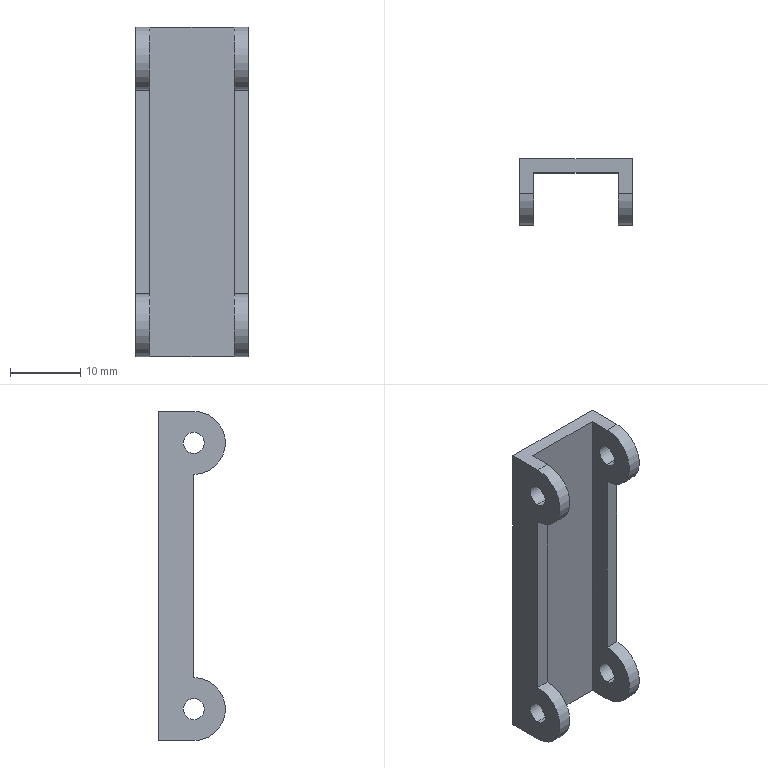Part | STEP file | Deraillieur Link Arms | 1 solid | 22 faces | box 16 x 9.5 x 47 mm | volume 2266 mm3 | cylinder 12 | plane 10 | commonest cylinder face diameters 3 x8 9 x4